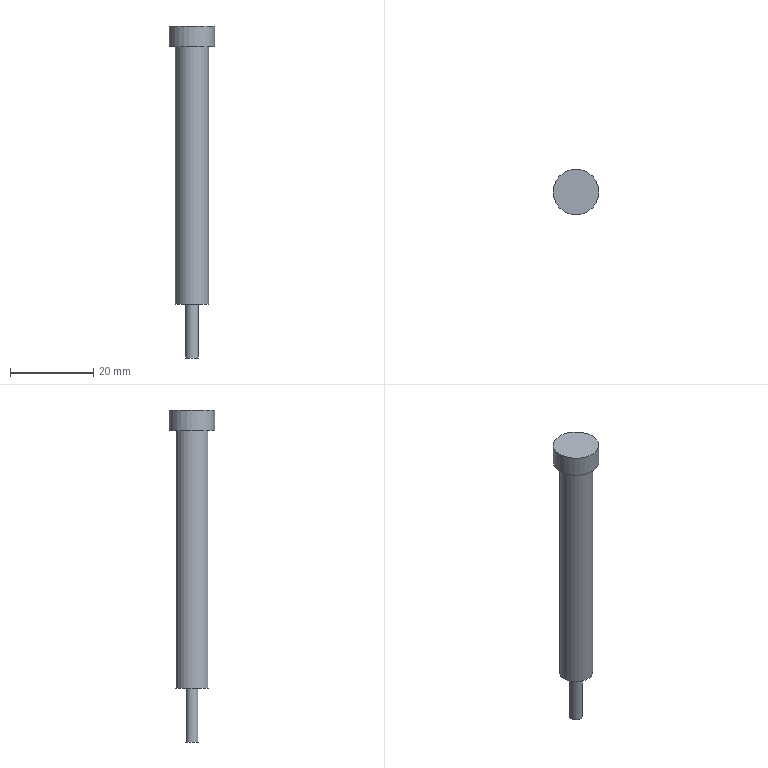Part | NX | features solid 2 | 1 solid | 7 faces | box 11 x 11 x 80 mm | volume 3690 mm3 | plane 4 | cylinder 3 | commonest cylinder face diameters 3.1 x1 8 x1 11 x1
STEP:
#1=CARTESIAN_POINT('',(-529.829,181.45,87.));
#2=VERTEX_POINT('',#1);
#3=CARTESIAN_POINT('',(-533.829,181.45,87.));
#4=DIRECTION('',(0.,0.,1.));
#5=DIRECTION('',(1.,0.,0.));
#6=AXIS2_PLACEMENT_3D('',#3,#4,#5);
#7=CIRCLE('',#6,4.);
#8=EDGE_CURVE('',#2,#2,#7,.T.);
#9=ORIENTED_EDGE('',*,*,#8,.T.);
#10=EDGE_LOOP('',(#9));
#11=FACE_BOUND('',#10,.T.);
#12=CARTESIAN_POINT('',(-529.829,181.45,149.));
#13=VERTEX_POINT('',#12);
#14=CARTESIAN_POINT('',(-533.829,181.45,149.));
#15=DIRECTION('',(0.,0.,1.));
#16=DIRECTION('',(1.,0.,0.));
#17=AXIS2_PLACEMENT_3D('',#14,#15,#16);
#18=CIRCLE('',#17,4.);
#19=EDGE_CURVE('',#13,#13,#18,.T.);
#20=ORIENTED_EDGE('',*,*,#19,.F.);
#21=EDGE_LOOP('',(#20));
#22=FACE_BOUND('',#21,.T.);
#23=CARTESIAN_POINT('',(-533.829,181.45,154.));
#24=DIRECTION('',(0.,0.,-1.));
#25=DIRECTION('',(-1.,0.,0.));
#26=AXIS2_PLACEMENT_3D('',#23,#24,#25);
#27=CYLINDRICAL_SURFACE('',#26,4.);
#28=ADVANCED_FACE('',(#11,#22),#27,.T.);
#29=CARTESIAN_POINT('',(-532.279,181.45,87.));
#30=VERTEX_POINT('',#29);
#31=CARTESIAN_POINT('',(-533.829,181.45,87.));
#32=DIRECTION('',(0.,0.,1.));
#33=DIRECTION('',(1.,0.,0.));
#34=AXIS2_PLACEMENT_3D('',#31,#32,#33);
#35=CIRCLE('',#34,1.55);
#36=EDGE_CURVE('',#30,#30,#35,.T.);
#37=ORIENTED_EDGE('',*,*,#36,.T.);
#38=EDGE_LOOP('',(#37));
#39=FACE_BOUND('',#38,.T.);
#40=ORIENTED_EDGE('',*,*,#8,.F.);
#41=EDGE_LOOP('',(#40));
#42=FACE_BOUND('',#41,.T.);
#43=CARTESIAN_POINT('',(-533.829,181.45,87.));
#44=DIRECTION('',(0.,0.,1.));
#45=DIRECTION('',(1.,0.,0.));
#46=AXIS2_PLACEMENT_3D('',#43,#44,#45);
#47=PLANE('',#46);
#48=ADVANCED_FACE('',(#39,#42),#47,.F.);
#49=CARTESIAN_POINT('',(-528.329,181.45,149.));
#50=VERTEX_POINT('',#49);
#51=CARTESIAN_POINT('',(-533.829,181.45,149.));
#52=DIRECTION('',(0.,0.,1.));
#53=DIRECTION('',(1.,0.,0.));
#54=AXIS2_PLACEMENT_3D('',#51,#52,#53);
#55=CIRCLE('',#54,5.5);
#56=EDGE_CURVE('',#50,#50,#55,.T.);
#57=ORIENTED_EDGE('',*,*,#56,.F.);
#58=EDGE_LOOP('',(#57));
#59=FACE_BOUND('',#58,.T.);
#60=ORIENTED_EDGE('',*,*,#19,.T.);
#61=EDGE_LOOP('',(#60));
#62=FACE_BOUND('',#61,.T.);
#63=CARTESIAN_POINT('',(-533.829,181.45,149.));
#64=DIRECTION('',(0.,0.,1.));
#65=DIRECTION('',(1.,0.,0.));
#66=AXIS2_PLACEMENT_3D('',#63,#64,#65);
#67=PLANE('',#66);
#68=ADVANCED_FACE('',(#59,#62),#67,.F.);
#69=ORIENTED_EDGE('',*,*,#56,.T.);
#70=EDGE_LOOP('',(#69));
#71=FACE_BOUND('',#70,.T.);
#72=CARTESIAN_POINT('',(-528.329,181.45,154.));
#73=VERTEX_POINT('',#72);
#74=CARTESIAN_POINT('',(-533.829,181.45,154.));
#75=DIRECTION('',(0.,0.,1.));
#76=DIRECTION('',(1.,0.,0.));
#77=AXIS2_PLACEMENT_3D('',#74,#75,#76);
#78=CIRCLE('',#77,5.5);
#79=EDGE_CURVE('',#73,#73,#78,.T.);
#80=ORIENTED_EDGE('',*,*,#79,.F.);
#81=EDGE_LOOP('',(#80));
#82=FACE_BOUND('',#81,.T.);
#83=CARTESIAN_POINT('',(-533.829,181.45,149.));
#84=DIRECTION('',(0.,0.,1.));
#85=DIRECTION('',(1.,0.,0.));
#86=AXIS2_PLACEMENT_3D('',#83,#84,#85);
#87=CYLINDRICAL_SURFACE('',#86,5.5);
#88=ADVANCED_FACE('',(#71,#82),#87,.T.);
#89=ORIENTED_EDGE('',*,*,#79,.T.);
#90=EDGE_LOOP('',(#89));
#91=FACE_BOUND('',#90,.T.);
#92=CARTESIAN_POINT('',(-533.829,181.45,154.));
#93=DIRECTION('',(0.,0.,1.));
#94=DIRECTION('',(1.,0.,0.));
#95=AXIS2_PLACEMENT_3D('',#92,#93,#94);
#96=PLANE('',#95);
#97=ADVANCED_FACE('',(#91),#96,.T.);
#98=CARTESIAN_POINT('',(-532.279,181.45,74.));
#99=VERTEX_POINT('',#98);
#100=CARTESIAN_POINT('',(-533.829,181.45,74.));
#101=DIRECTION('',(0.,0.,1.));
#102=DIRECTION('',(1.,0.,0.));
#103=AXIS2_PLACEMENT_3D('',#100,#101,#102);
#104=CIRCLE('',#103,1.55);
#105=EDGE_CURVE('',#99,#99,#104,.T.);
#106=ORIENTED_EDGE('',*,*,#105,.T.);
#107=EDGE_LOOP('',(#106));
#108=FACE_BOUND('',#107,.T.);
#109=ORIENTED_EDGE('',*,*,#36,.F.);
#110=EDGE_LOOP('',(#109));
#111=FACE_BOUND('',#110,.T.);
#112=CARTESIAN_POINT('',(-533.829,181.45,74.));
#113=DIRECTION('',(0.,0.,1.));
#114=DIRECTION('',(1.,0.,0.));
#115=AXIS2_PLACEMENT_3D('',#112,#113,#114);
#116=CYLINDRICAL_SURFACE('',#115,1.55);
#117=ADVANCED_FACE('',(#108,#111),#116,.T.);
#118=ORIENTED_EDGE('',*,*,#105,.F.);
#119=EDGE_LOOP('',(#118));
#120=FACE_BOUND('',#119,.T.);
#121=CARTESIAN_POINT('',(-533.829,181.45,74.));
#122=DIRECTION('',(0.,0.,1.));
#123=DIRECTION('',(1.,0.,0.));
#124=AXIS2_PLACEMENT_3D('',#121,#122,#123);
#125=PLANE('',#124);
#126=ADVANCED_FACE('',(#120),#125,.F.);
#127=CLOSED_SHELL('',(#28,#48,#68,#88,#97,#117,#126));
#128=MANIFOLD_SOLID_BREP('',#127);
#129=(LENGTH_UNIT()NAMED_UNIT(*)SI_UNIT(.MILLI.,.METRE.));
#130=UNCERTAINTY_MEASURE_WITH_UNIT(LENGTH_MEASURE(0.00001),#129,'','');
#131=(NAMED_UNIT(*)PLANE_ANGLE_UNIT()SI_UNIT($,.RADIAN.));
#132=(NAMED_UNIT(*)SI_UNIT($,.STERADIAN.)SOLID_ANGLE_UNIT());
#133=(GEOMETRIC_REPRESENTATION_CONTEXT(3)GLOBAL_UNCERTAINTY_ASSIGNED_CONTEXT((#130))GLOBAL_UNIT_ASSIGNED_CONTEXT((#129,#131,#132))REPRESENTATION_CONTEXT('',''));
#134=ADVANCED_BREP_SHAPE_REPRESENTATION('',(#128),#133);